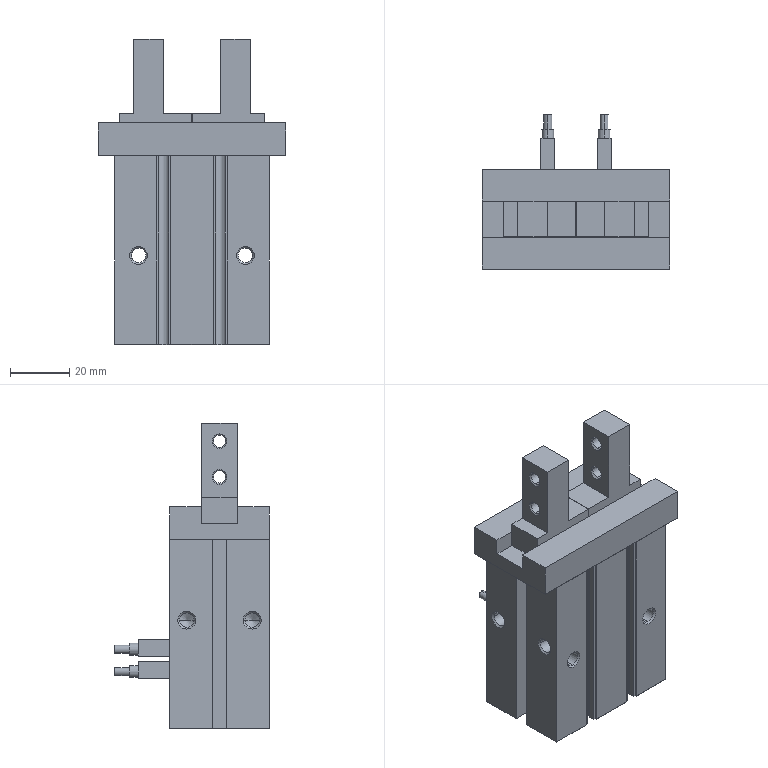Part | STEP file | Bag feed finger cylinder MHZ2-25D-F8N (19.3) | 1 solid | 246 faces | box 63 x 52.1 x 102.7 mm | volume 124711 mm3 | plane 144 | cylinder 58 | cone 44 | commonest cylinder face diameters 4.92 x16 4 x12 4.02 x12 4.13 x8 2.7 x4 4.48 x4